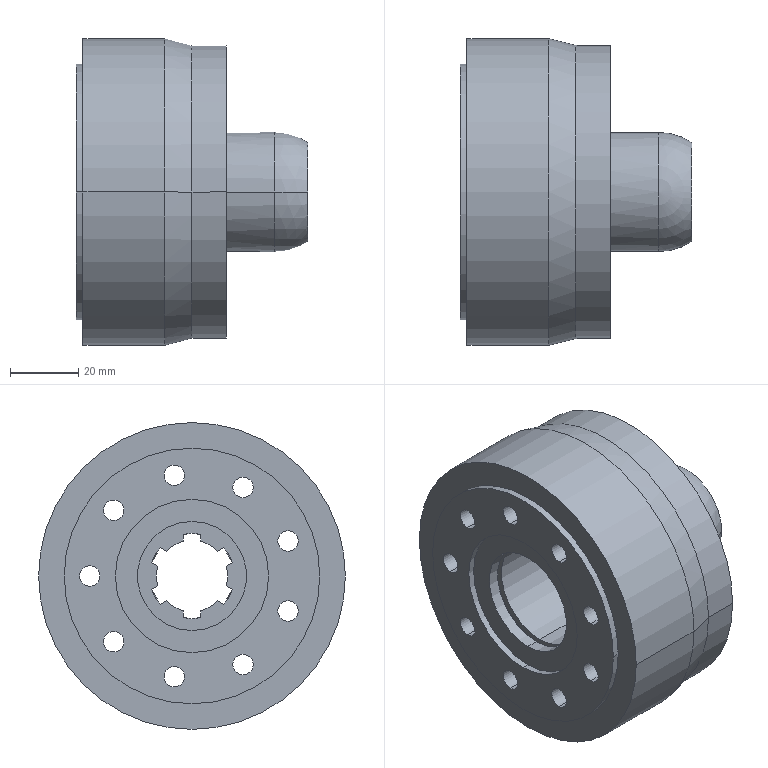Part | SolidWorks | features Chamfer 1, CirPattern 1, HoleWzd 1, ICE 1, RevCut 1, Revolution 1 | 1 solid | 135 faces | box 68 x 90 x 90 mm | volume 185813 mm3 | cylinder 60 | cone 38 | plane 35 | sphere 2 | commonest cylinder face diameters 6 x18 15 x18 21 x6 32 x4 25 x2 35 x2